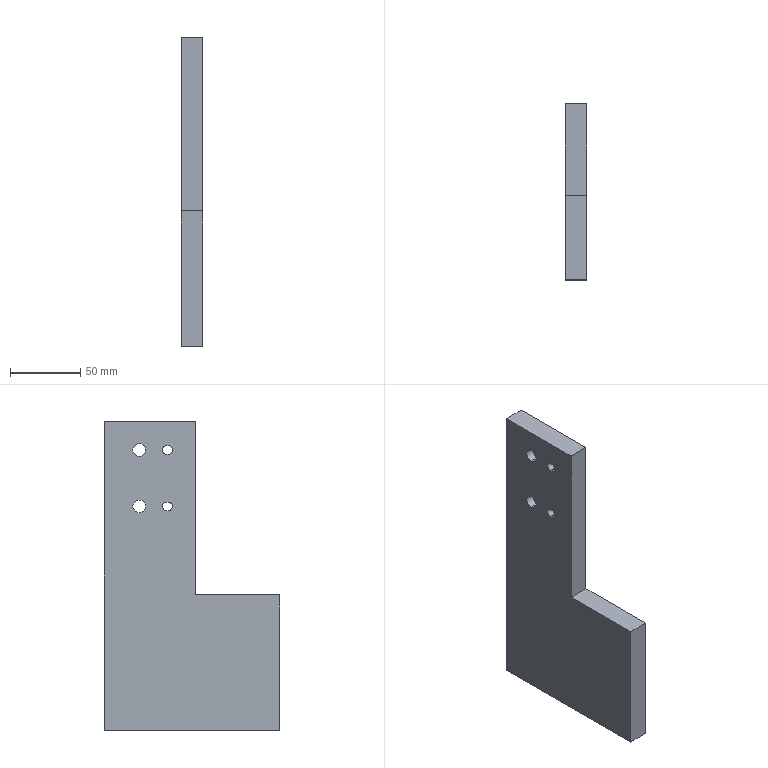Part | SolidWorks | features HoleWzd 6, Fillet 2, ICE 2, Chamfer 1, Extrusion 1 | 1 solid | 34 faces | box 15 x 125 x 219 mm | volume 294597 mm3 | cylinder 16 | plane 14 | cone 4 | commonest cylinder face diameters 4.2 x4 6 x4 9 x4 15 x4
STEP:
#1=CARTESIAN_POINT('',(2.6,-83.5,-42.9));
#2=VERTEX_POINT('',#1);
#3=CARTESIAN_POINT('',(2.6,-83.5,-47.1));
#4=VERTEX_POINT('',#3);
#5=CARTESIAN_POINT('',(2.6,-83.5,-45.));
#6=DIRECTION('',(1.,0.,0.));
#7=DIRECTION('',(0.,0.,-1.));
#8=AXIS2_PLACEMENT_3D('',#5,#6,#7);
#9=CIRCLE('',#8,2.1);
#10=EDGE_CURVE('',#2,#4,#9,.T.);
#11=ORIENTED_EDGE('',*,*,#10,.F.);
#12=CARTESIAN_POINT('',(15.,-83.5,-42.9));
#13=VERTEX_POINT('',#12);
#14=CARTESIAN_POINT('',(15.,-83.5,-42.9));
#15=DIRECTION('',(1.,0.,0.));
#16=VECTOR('',#15,1000.);
#17=LINE('',#14,#16);
#18=EDGE_CURVE('',#2,#13,#17,.T.);
#19=ORIENTED_EDGE('',*,*,#18,.T.);
#20=CARTESIAN_POINT('',(15.,-83.5,-47.1));
#21=VERTEX_POINT('',#20);
#22=CARTESIAN_POINT('',(15.,-83.5,-45.));
#23=DIRECTION('',(1.,0.,0.));
#24=DIRECTION('',(0.,0.,-1.));
#25=AXIS2_PLACEMENT_3D('',#22,#23,#24);
#26=CIRCLE('',#25,2.1);
#27=EDGE_CURVE('',#13,#21,#26,.T.);
#28=ORIENTED_EDGE('',*,*,#27,.T.);
#29=CARTESIAN_POINT('',(15.,-83.5,-47.1));
#30=DIRECTION('',(1.,0.,0.));
#31=VECTOR('',#30,1000.);
#32=LINE('',#29,#31);
#33=EDGE_CURVE('',#4,#21,#32,.T.);
#34=ORIENTED_EDGE('',*,*,#33,.F.);
#35=EDGE_LOOP('',(#11,#19,#28,#34));
#36=FACE_OUTER_BOUND('',#35,.T.);
#37=CARTESIAN_POINT('',(15.,-83.5,-45.));
#38=DIRECTION('',(1.,0.,0.));
#39=DIRECTION('',(0.,0.,-1.));
#40=AXIS2_PLACEMENT_3D('',#37,#38,#39);
#41=CYLINDRICAL_SURFACE('',#40,2.1);
#42=ADVANCED_FACE('',(#36),#41,.F.);
#43=CARTESIAN_POINT('',(1.338,-83.5,-45.));
#44=VERTEX_POINT('',#43);
#45=CARTESIAN_POINT('',(2.6,-83.5,-47.1));
#46=DIRECTION('',(0.515,0.,-0.8572));
#47=VECTOR('',#46,1000.);
#48=LINE('',#45,#47);
#49=EDGE_CURVE('',#44,#4,#48,.T.);
#50=ORIENTED_EDGE('',*,*,#49,.F.);
#51=CARTESIAN_POINT('',(2.6,-83.5,-42.9));
#52=DIRECTION('',(0.515,0.,0.8572));
#53=VECTOR('',#52,1000.);
#54=LINE('',#51,#53);
#55=EDGE_CURVE('',#44,#2,#54,.T.);
#56=ORIENTED_EDGE('',*,*,#55,.T.);
#57=ORIENTED_EDGE('',*,*,#10,.T.);
#58=EDGE_LOOP('',(#50,#56,#57));
#59=FACE_OUTER_BOUND('',#58,.T.);
#60=CARTESIAN_POINT('',(2.6,-83.5,-45.));
#61=DIRECTION('',(1.,0.,0.));
#62=DIRECTION('',(0.,0.,-1.));
#63=AXIS2_PLACEMENT_3D('',#60,#61,#62);
#64=CONICAL_SURFACE('',#63,2.1,1.03);
#65=ADVANCED_FACE('',(#59),#64,.F.);
#66=CARTESIAN_POINT('',(2.6,-83.5,-97.9));
#67=VERTEX_POINT('',#66);
#68=CARTESIAN_POINT('',(2.6,-83.5,-102.1));
#69=VERTEX_POINT('',#68);
#70=CARTESIAN_POINT('',(2.6,-83.5,-100.));
#71=DIRECTION('',(1.,0.,0.));
#72=DIRECTION('',(0.,0.,-1.));
#73=AXIS2_PLACEMENT_3D('',#70,#71,#72);
#74=CIRCLE('',#73,2.1);
#75=EDGE_CURVE('',#67,#69,#74,.T.);
#76=ORIENTED_EDGE('',*,*,#75,.F.);
#77=CARTESIAN_POINT('',(15.,-83.5,-97.9));
#78=VERTEX_POINT('',#77);
#79=CARTESIAN_POINT('',(15.,-83.5,-97.9));
#80=DIRECTION('',(1.,0.,0.));
#81=VECTOR('',#80,1000.);
#82=LINE('',#79,#81);
#83=EDGE_CURVE('',#67,#78,#82,.T.);
#84=ORIENTED_EDGE('',*,*,#83,.T.);
#85=CARTESIAN_POINT('',(15.,-83.5,-102.1));
#86=VERTEX_POINT('',#85);
#87=CARTESIAN_POINT('',(15.,-83.5,-100.));
#88=DIRECTION('',(1.,0.,0.));
#89=DIRECTION('',(0.,0.,-1.));
#90=AXIS2_PLACEMENT_3D('',#87,#88,#89);
#91=CIRCLE('',#90,2.1);
#92=EDGE_CURVE('',#78,#86,#91,.T.);
#93=ORIENTED_EDGE('',*,*,#92,.T.);
#94=CARTESIAN_POINT('',(15.,-83.5,-102.1));
#95=DIRECTION('',(1.,0.,0.));
#96=VECTOR('',#95,1000.);
#97=LINE('',#94,#96);
#98=EDGE_CURVE('',#69,#86,#97,.T.);
#99=ORIENTED_EDGE('',*,*,#98,.F.);
#100=EDGE_LOOP('',(#76,#84,#93,#99));
#101=FACE_OUTER_BOUND('',#100,.T.);
#102=CARTESIAN_POINT('',(15.,-83.5,-100.));
#103=DIRECTION('',(1.,0.,0.));
#104=DIRECTION('',(0.,0.,-1.));
#105=AXIS2_PLACEMENT_3D('',#102,#103,#104);
#106=CYLINDRICAL_SURFACE('',#105,2.1);
#107=ADVANCED_FACE('',(#101),#106,.F.);
#108=CARTESIAN_POINT('',(1.338,-83.5,-100.));
#109=VERTEX_POINT('',#108);
#110=CARTESIAN_POINT('',(2.6,-83.5,-102.1));
#111=DIRECTION('',(0.515,0.,-0.8572));
#112=VECTOR('',#111,1000.);
#113=LINE('',#110,#112);
#114=EDGE_CURVE('',#109,#69,#113,.T.);
#115=ORIENTED_EDGE('',*,*,#114,.F.);
#116=CARTESIAN_POINT('',(2.6,-83.5,-97.9));
#117=DIRECTION('',(0.515,0.,0.8572));
#118=VECTOR('',#117,1000.);
#119=LINE('',#116,#118);
#120=EDGE_CURVE('',#109,#67,#119,.T.);
#121=ORIENTED_EDGE('',*,*,#120,.T.);
#122=ORIENTED_EDGE('',*,*,#75,.T.);
#123=EDGE_LOOP('',(#115,#121,#122));
#124=FACE_OUTER_BOUND('',#123,.T.);
#125=CARTESIAN_POINT('',(2.6,-83.5,-100.));
#126=DIRECTION('',(1.,0.,0.));
#127=DIRECTION('',(0.,0.,-1.));
#128=AXIS2_PLACEMENT_3D('',#125,#126,#127);
#129=CONICAL_SURFACE('',#128,2.1,1.03);
#130=ADVANCED_FACE('',(#124),#129,.F.);
#131=CARTESIAN_POINT('',(6.,7.5,97.));
#132=VERTEX_POINT('',#131);
#133=CARTESIAN_POINT('',(6.,7.5,82.));
#134=VERTEX_POINT('',#133);
#135=CARTESIAN_POINT('',(6.,7.5,89.5));
#136=DIRECTION('',(1.,0.,0.));
#137=DIRECTION('',(0.,0.,-1.));
#138=AXIS2_PLACEMENT_3D('',#135,#136,#137);
#139=CIRCLE('',#138,7.5);
#140=EDGE_CURVE('',#132,#134,#139,.T.);
#141=ORIENTED_EDGE('',*,*,#140,.F.);
#142=CARTESIAN_POINT('',(15.,7.5,97.));
#143=VERTEX_POINT('',#142);
#144=CARTESIAN_POINT('',(15.,7.5,97.));
#145=DIRECTION('',(1.,0.,0.));
#146=VECTOR('',#145,1000.);
#147=LINE('',#144,#146);
#148=EDGE_CURVE('',#132,#143,#147,.T.);
#149=ORIENTED_EDGE('',*,*,#148,.T.);
#150=CARTESIAN_POINT('',(15.,7.5,82.));
#151=VERTEX_POINT('',#150);
#152=CARTESIAN_POINT('',(15.,7.5,89.5));
#153=DIRECTION('',(1.,0.,0.));
#154=DIRECTION('',(0.,0.,-1.));
#155=AXIS2_PLACEMENT_3D('',#152,#153,#154);
#156=CIRCLE('',#155,7.5);
#157=EDGE_CURVE('',#143,#151,#156,.T.);
#158=ORIENTED_EDGE('',*,*,#157,.T.);
#159=CARTESIAN_POINT('',(15.,7.5,82.));
#160=DIRECTION('',(1.,0.,0.));
#161=VECTOR('',#160,1000.);
#162=LINE('',#159,#161);
#163=EDGE_CURVE('',#134,#151,#162,.T.);
#164=ORIENTED_EDGE('',*,*,#163,.F.);
#165=EDGE_LOOP('',(#141,#149,#158,#164));
#166=FACE_OUTER_BOUND('',#165,.T.);
#167=CARTESIAN_POINT('',(15.,7.5,89.5));
#168=DIRECTION('',(1.,0.,0.));
#169=DIRECTION('',(0.,0.,-1.));
#170=AXIS2_PLACEMENT_3D('',#167,#168,#169);
#171=CYLINDRICAL_SURFACE('',#170,7.5);
#172=ADVANCED_FACE('',(#166),#171,.F.);
#173=CARTESIAN_POINT('',(0.,7.5,94.));
#174=VERTEX_POINT('',#173);
#175=CARTESIAN_POINT('',(0.,7.5,85.));
#176=VERTEX_POINT('',#175);
#177=CARTESIAN_POINT('',(0.,7.5,89.5));
#178=DIRECTION('',(1.,0.,0.));
#179=DIRECTION('',(0.,0.,-1.));
#180=AXIS2_PLACEMENT_3D('',#177,#178,#179);
#181=CIRCLE('',#180,4.5);
#182=EDGE_CURVE('',#174,#176,#181,.T.);
#183=ORIENTED_EDGE('',*,*,#182,.F.);
#184=CARTESIAN_POINT('',(6.,7.5,94.));
#185=VERTEX_POINT('',#184);
#186=CARTESIAN_POINT('',(15.,7.5,94.));
#187=DIRECTION('',(1.,0.,0.));
#188=VECTOR('',#187,1000.);
#189=LINE('',#186,#188);
#190=EDGE_CURVE('',#174,#185,#189,.T.);
#191=ORIENTED_EDGE('',*,*,#190,.T.);
#192=CARTESIAN_POINT('',(6.,7.5,85.));
#193=VERTEX_POINT('',#192);
#194=CARTESIAN_POINT('',(6.,7.5,89.5));
#195=DIRECTION('',(1.,0.,0.));
#196=DIRECTION('',(0.,0.,-1.));
#197=AXIS2_PLACEMENT_3D('',#194,#195,#196);
#198=CIRCLE('',#197,4.5);
#199=EDGE_CURVE('',#185,#193,#198,.T.);
#200=ORIENTED_EDGE('',*,*,#199,.T.);
#201=CARTESIAN_POINT('',(15.,7.5,85.));
#202=DIRECTION('',(1.,0.,0.));
#203=VECTOR('',#202,1000.);
#204=LINE('',#201,#203);
#205=EDGE_CURVE('',#176,#193,#204,.T.);
#206=ORIENTED_EDGE('',*,*,#205,.F.);
#207=EDGE_LOOP('',(#183,#191,#200,#206));
#208=FACE_OUTER_BOUND('',#207,.T.);
#209=CARTESIAN_POINT('',(15.,7.5,89.5));
#210=DIRECTION('',(1.,0.,0.));
#211=DIRECTION('',(0.,0.,-1.));
#212=AXIS2_PLACEMENT_3D('',#209,#210,#211);
#213=CYLINDRICAL_SURFACE('',#212,4.5);
#214=ADVANCED_FACE('',(#208),#213,.F.);
#215=CARTESIAN_POINT('',(6.,7.5,57.));
#216=VERTEX_POINT('',#215);
#217=CARTESIAN_POINT('',(6.,7.5,42.));
#218=VERTEX_POINT('',#217);
#219=CARTESIAN_POINT('',(6.,7.5,49.5));
#220=DIRECTION('',(1.,0.,0.));
#221=DIRECTION('',(0.,0.,-1.));
#222=AXIS2_PLACEMENT_3D('',#219,#220,#221);
#223=CIRCLE('',#222,7.5);
#224=EDGE_CURVE('',#216,#218,#223,.T.);
#225=ORIENTED_EDGE('',*,*,#224,.F.);
#226=CARTESIAN_POINT('',(15.,7.5,57.));
#227=VERTEX_POINT('',#226);
#228=CARTESIAN_POINT('',(15.,7.5,57.));
#229=DIRECTION('',(1.,0.,0.));
#230=VECTOR('',#229,1000.);
#231=LINE('',#228,#230);
#232=EDGE_CURVE('',#216,#227,#231,.T.);
#233=ORIENTED_EDGE('',*,*,#232,.T.);
#234=CARTESIAN_POINT('',(15.,7.5,42.));
#235=VERTEX_POINT('',#234);
#236=CARTESIAN_POINT('',(15.,7.5,49.5));
#237=DIRECTION('',(1.,0.,0.));
#238=DIRECTION('',(0.,0.,-1.));
#239=AXIS2_PLACEMENT_3D('',#236,#237,#238);
#240=CIRCLE('',#239,7.5);
#241=EDGE_CURVE('',#227,#235,#240,.T.);
#242=ORIENTED_EDGE('',*,*,#241,.T.);
#243=CARTESIAN_POINT('',(15.,7.5,42.));
#244=DIRECTION('',(1.,0.,0.));
#245=VECTOR('',#244,1000.);
#246=LINE('',#243,#245);
#247=EDGE_CURVE('',#218,#235,#246,.T.);
#248=ORIENTED_EDGE('',*,*,#247,.F.);
#249=EDGE_LOOP('',(#225,#233,#242,#248));
#250=FACE_OUTER_BOUND('',#249,.T.);
#251=CARTESIAN_POINT('',(15.,7.5,49.5));
#252=DIRECTION('',(1.,0.,0.));
#253=DIRECTION('',(0.,0.,-1.));
#254=AXIS2_PLACEMENT_3D('',#251,#252,#253);
#255=CYLINDRICAL_SURFACE('',#254,7.5);
#256=ADVANCED_FACE('',(#250),#255,.F.);
#257=CARTESIAN_POINT('',(0.,7.5,54.));
#258=VERTEX_POINT('',#257);
#259=CARTESIAN_POINT('',(0.,7.5,45.));
#260=VERTEX_POINT('',#259);
#261=CARTESIAN_POINT('',(0.,7.5,49.5));
#262=DIRECTION('',(1.,0.,0.));
#263=DIRECTION('',(0.,0.,-1.));
#264=AXIS2_PLACEMENT_3D('',#261,#262,#263);
#265=CIRCLE('',#264,4.5);
#266=EDGE_CURVE('',#258,#260,#265,.T.);
#267=ORIENTED_EDGE('',*,*,#266,.F.);
#268=CARTESIAN_POINT('',(6.,7.5,54.));
#269=VERTEX_POINT('',#268);
#270=CARTESIAN_POINT('',(15.,7.5,54.));
#271=DIRECTION('',(1.,0.,0.));
#272=VECTOR('',#271,1000.);
#273=LINE('',#270,#272);
#274=EDGE_CURVE('',#258,#269,#273,.T.);
#275=ORIENTED_EDGE('',*,*,#274,.T.);
#276=CARTESIAN_POINT('',(6.,7.5,45.));
#277=VERTEX_POINT('',#276);
#278=CARTESIAN_POINT('',(6.,7.5,49.5));
#279=DIRECTION('',(1.,0.,0.));
#280=DIRECTION('',(0.,0.,-1.));
#281=AXIS2_PLACEMENT_3D('',#278,#279,#280);
#282=CIRCLE('',#281,4.5);
#283=EDGE_CURVE('',#269,#277,#282,.T.);
#284=ORIENTED_EDGE('',*,*,#283,.T.);
#285=CARTESIAN_POINT('',(15.,7.5,45.));
#286=DIRECTION('',(1.,0.,0.));
#287=VECTOR('',#286,1000.);
#288=LINE('',#285,#287);
#289=EDGE_CURVE('',#260,#277,#288,.T.);
#290=ORIENTED_EDGE('',*,*,#289,.F.);
#291=EDGE_LOOP('',(#267,#275,#284,#290));
#292=FACE_OUTER_BOUND('',#291,.T.);
#293=CARTESIAN_POINT('',(15.,7.5,49.5));
#294=DIRECTION('',(1.,0.,0.));
#295=DIRECTION('',(0.,0.,-1.));
#296=AXIS2_PLACEMENT_3D('',#293,#294,#295);
#297=CYLINDRICAL_SURFACE('',#296,4.5);
#298=ADVANCED_FACE('',(#292),#297,.F.);
#299=CARTESIAN_POINT('',(15.,-32.5,-13.5));
#300=VERTEX_POINT('',#299);
#301=CARTESIAN_POINT('',(0.,-32.5,-13.5));
#302=VERTEX_POINT('',#301);
#303=CARTESIAN_POINT('',(0.,-32.5,-13.5));
#304=DIRECTION('',(-1.,0.,0.));
#305=VECTOR('',#304,1000.);
#306=LINE('',#303,#305);
#307=EDGE_CURVE('',#300,#302,#306,.T.);
#308=ORIENTED_EDGE('',*,*,#307,.F.);
#309=CARTESIAN_POINT('',(15.,-32.5,109.5));
#310=VERTEX_POINT('',#309);
#311=CARTESIAN_POINT('',(15.,-32.5,109.5));
#312=DIRECTION('',(0.,0.,-1.));
#313=VECTOR('',#312,1000.);
#314=LINE('',#311,#313);
#315=EDGE_CURVE('',#310,#300,#314,.T.);
#316=ORIENTED_EDGE('',*,*,#315,.F.);
#317=CARTESIAN_POINT('',(0.,-32.5,109.5));
#318=VERTEX_POINT('',#317);
#319=CARTESIAN_POINT('',(15.,-32.5,109.5));
#320=DIRECTION('',(-1.,0.,0.));
#321=VECTOR('',#320,1000.);
#322=LINE('',#319,#321);
#323=EDGE_CURVE('',#310,#318,#322,.T.);
#324=ORIENTED_EDGE('',*,*,#323,.T.);
#325=CARTESIAN_POINT('',(0.,-32.5,109.5));
#326=DIRECTION('',(0.,0.,-1.));
#327=VECTOR('',#326,1000.);
#328=LINE('',#325,#327);
#329=EDGE_CURVE('',#318,#302,#328,.T.);
#330=ORIENTED_EDGE('',*,*,#329,.T.);
#331=EDGE_LOOP('',(#308,#316,#324,#330));
#332=FACE_OUTER_BOUND('',#331,.T.);
#333=CARTESIAN_POINT('',(15.,-32.5,109.5));
#334=DIRECTION('',(0.,1.,0.));
#335=DIRECTION('',(0.,0.,1.));
#336=AXIS2_PLACEMENT_3D('',#333,#334,#335);
#337=PLANE('',#336);
#338=ADVANCED_FACE('',(#332),#337,.F.);
#339=CARTESIAN_POINT('',(15.,-83.5,-45.));
#340=DIRECTION('',(1.,0.,0.));
#341=DIRECTION('',(0.,0.,-1.));
#342=AXIS2_PLACEMENT_3D('',#339,#340,#341);
#343=CIRCLE('',#342,2.1);
#344=EDGE_CURVE('',#21,#13,#343,.T.);
#345=ORIENTED_EDGE('',*,*,#344,.F.);
#346=ORIENTED_EDGE('',*,*,#27,.F.);
#347=EDGE_LOOP('',(#345,#346));
#348=FACE_BOUND('',#347,.T.);
#349=CARTESIAN_POINT('',(15.,-83.5,-100.));
#350=DIRECTION('',(1.,0.,0.));
#351=DIRECTION('',(0.,0.,-1.));
#352=AXIS2_PLACEMENT_3D('',#349,#350,#351);
#353=CIRCLE('',#352,2.1);
#354=EDGE_CURVE('',#86,#78,#353,.T.);
#355=ORIENTED_EDGE('',*,*,#354,.F.);
#356=ORIENTED_EDGE('',*,*,#92,.F.);
#357=EDGE_LOOP('',(#355,#356));
#358=FACE_BOUND('',#357,.T.);
#359=CARTESIAN_POINT('',(15.,-92.5,-109.5));
#360=VERTEX_POINT('',#359);
#361=CARTESIAN_POINT('',(15.,32.5,-109.5));
#362=VERTEX_POINT('',#361);
#363=CARTESIAN_POINT('',(15.,-32.5,-109.5));
#364=DIRECTION('',(0.,1.,0.));
#365=VECTOR('',#364,1000.);
#366=LINE('',#363,#365);
#367=EDGE_CURVE('',#360,#362,#366,.T.);
#368=ORIENTED_EDGE('',*,*,#367,.T.);
#369=CARTESIAN_POINT('',(15.,32.5,109.5));
#370=VERTEX_POINT('',#369);
#371=CARTESIAN_POINT('',(15.,32.5,109.5));
#372=DIRECTION('',(0.,0.,1.));
#373=VECTOR('',#372,1000.);
#374=LINE('',#371,#373);
#375=EDGE_CURVE('',#362,#370,#374,.T.);
#376=ORIENTED_EDGE('',*,*,#375,.T.);
#377=CARTESIAN_POINT('',(15.,-32.5,109.5));
#378=DIRECTION('',(0.,-1.,0.));
#379=VECTOR('',#378,1000.);
#380=LINE('',#377,#379);
#381=EDGE_CURVE('',#370,#310,#380,.T.);
#382=ORIENTED_EDGE('',*,*,#381,.T.);
#383=ORIENTED_EDGE('',*,*,#315,.T.);
#384=CARTESIAN_POINT('',(15.,-92.5,-13.5));
#385=VERTEX_POINT('',#384);
#386=CARTESIAN_POINT('',(15.,-92.5,-13.5));
#387=DIRECTION('',(0.,1.,0.));
#388=VECTOR('',#387,1000.);
#389=LINE('',#386,#388);
#390=EDGE_CURVE('',#385,#300,#389,.T.);
#391=ORIENTED_EDGE('',*,*,#390,.F.);
#392=CARTESIAN_POINT('',(15.,-92.5,-109.5));
#393=DIRECTION('',(0.,0.,1.));
#394=VECTOR('',#393,1000.);
#395=LINE('',#392,#394);
#396=EDGE_CURVE('',#360,#385,#395,.T.);
#397=ORIENTED_EDGE('',*,*,#396,.F.);
#398=EDGE_LOOP('',(#368,#376,#382,#383,#391,#397));
#399=FACE_OUTER_BOUND('',#398,.T.);
#400=CARTESIAN_POINT('',(15.,7.5,49.5));
#401=DIRECTION('',(1.,0.,0.));
#402=DIRECTION('',(0.,0.,-1.));
#403=AXIS2_PLACEMENT_3D('',#400,#401,#402);
#404=CIRCLE('',#403,7.5);
#405=EDGE_CURVE('',#235,#227,#404,.T.);
#406=ORIENTED_EDGE('',*,*,#405,.F.);
#407=ORIENTED_EDGE('',*,*,#241,.F.);
#408=EDGE_LOOP('',(#406,#407));
#409=FACE_BOUND('',#408,.T.);
#410=CARTESIAN_POINT('',(15.,7.5,89.5));
#411=DIRECTION('',(1.,0.,0.));
#412=DIRECTION('',(0.,0.,-1.));
#413=AXIS2_PLACEMENT_3D('',#410,#411,#412);
#414=CIRCLE('',#413,7.5);
#415=EDGE_CURVE('',#151,#143,#414,.T.);
#416=ORIENTED_EDGE('',*,*,#415,.F.);
#417=ORIENTED_EDGE('',*,*,#157,.F.);
#418=EDGE_LOOP('',(#416,#417));
#419=FACE_BOUND('',#418,.T.);
#420=CARTESIAN_POINT('',(15.,-13.,52.5));
#421=VERTEX_POINT('',#420);
#422=CARTESIAN_POINT('',(15.,-13.,46.5));
#423=VERTEX_POINT('',#422);
#424=CARTESIAN_POINT('',(15.,-13.,49.5));
#425=DIRECTION('',(1.,0.,0.));
#426=DIRECTION('',(0.,0.,-1.));
#427=AXIS2_PLACEMENT_3D('',#424,#425,#426);
#428=CIRCLE('',#427,3.);
#429=EDGE_CURVE('',#421,#423,#428,.T.);
#430=ORIENTED_EDGE('',*,*,#429,.F.);
#431=CARTESIAN_POINT('',(15.,-12.,52.5));
#432=VERTEX_POINT('',#431);
#433=CARTESIAN_POINT('',(15.,-13.,52.5));
#434=DIRECTION('',(0.,1.,0.));
#435=VECTOR('',#434,1000.);
#436=LINE('',#433,#435);
#437=EDGE_CURVE('',#421,#432,#436,.T.);
#438=ORIENTED_EDGE('',*,*,#437,.T.);
#439=CARTESIAN_POINT('',(15.,-12.,46.5));
#440=VERTEX_POINT('',#439);
#441=CARTESIAN_POINT('',(15.,-12.,49.5));
#442=DIRECTION('',(1.,0.,0.));
#443=DIRECTION('',(0.,0.,-1.));
#444=AXIS2_PLACEMENT_3D('',#441,#442,#443);
#445=CIRCLE('',#444,3.);
#446=EDGE_CURVE('',#440,#432,#445,.T.);
#447=ORIENTED_EDGE('',*,*,#446,.F.);
#448=CARTESIAN_POINT('',(15.,-13.,46.5));
#449=DIRECTION('',(0.,1.,0.));
#450=VECTOR('',#449,1000.);
#451=LINE('',#448,#450);
#452=EDGE_CURVE('',#423,#440,#451,.T.);
#453=ORIENTED_EDGE('',*,*,#452,.F.);
#454=EDGE_LOOP('',(#430,#438,#447,#453));
#455=FACE_BOUND('',#454,.T.);
#456=CARTESIAN_POINT('',(15.,-12.,86.5));
#457=VERTEX_POINT('',#456);
#458=CARTESIAN_POINT('',(15.,-12.,92.5));
#459=VERTEX_POINT('',#458);
#460=CARTESIAN_POINT('',(15.,-12.,89.5));
#461=DIRECTION('',(1.,0.,0.));
#462=DIRECTION('',(0.,0.,-1.));
#463=AXIS2_PLACEMENT_3D('',#460,#461,#462);
#464=CIRCLE('',#463,3.);
#465=EDGE_CURVE('',#457,#459,#464,.T.);
#466=ORIENTED_EDGE('',*,*,#465,.F.);
#467=CARTESIAN_POINT('',(15.,-13.,86.5));
#468=VERTEX_POINT('',#467);
#469=CARTESIAN_POINT('',(15.,-13.,86.5));
#470=DIRECTION('',(0.,1.,0.));
#471=VECTOR('',#470,1000.);
#472=LINE('',#469,#471);
#473=EDGE_CURVE('',#468,#457,#472,.T.);
#474=ORIENTED_EDGE('',*,*,#473,.F.);
#475=CARTESIAN_POINT('',(15.,-13.,92.5));
#476=VERTEX_POINT('',#475);
#477=CARTESIAN_POINT('',(15.,-13.,89.5));
#478=DIRECTION('',(1.,0.,0.));
#479=DIRECTION('',(0.,0.,-1.));
#480=AXIS2_PLACEMENT_3D('',#477,#478,#479);
#481=CIRCLE('',#480,3.);
#482=EDGE_CURVE('',#476,#468,#481,.T.);
#483=ORIENTED_EDGE('',*,*,#482,.F.);
#484=CARTESIAN_POINT('',(15.,-13.,92.5));
#485=DIRECTION('',(0.,1.,0.));
#486=VECTOR('',#485,1000.);
#487=LINE('',#484,#486);
#488=EDGE_CURVE('',#476,#459,#487,.T.);
#489=ORIENTED_EDGE('',*,*,#488,.T.);
#490=EDGE_LOOP('',(#466,#474,#483,#489));
#491=FACE_BOUND('',#490,.T.);
#492=CARTESIAN_POINT('',(15.,0.,0.));
#493=DIRECTION('',(-1.,0.,0.));
#494=DIRECTION('',(0.,0.,1.));
#495=AXIS2_PLACEMENT_3D('',#492,#493,#494);
#496=PLANE('',#495);
#497=ADVANCED_FACE('',(#348,#358,#399,#409,#419,#455,#491),#496,.F.);
#498=CARTESIAN_POINT('',(0.,-13.,46.5));
#499=VERTEX_POINT('',#498);
#500=CARTESIAN_POINT('',(0.,-12.,46.5));
#501=VERTEX_POINT('',#500);
#502=CARTESIAN_POINT('',(0.,-13.,46.5));
#503=DIRECTION('',(0.,1.,0.));
#504=VECTOR('',#503,1000.);
#505=LINE('',#502,#504);
#506=EDGE_CURVE('',#499,#501,#505,.T.);
#507=ORIENTED_EDGE('',*,*,#506,.T.);
#508=CARTESIAN_POINT('',(0.,-12.,52.5));
#509=VERTEX_POINT('',#508);
#510=CARTESIAN_POINT('',(0.,-12.,49.5));
#511=DIRECTION('',(1.,0.,0.));
#512=DIRECTION('',(0.,0.,-1.));
#513=AXIS2_PLACEMENT_3D('',#510,#511,#512);
#514=CIRCLE('',#513,3.);
#515=EDGE_CURVE('',#501,#509,#514,.T.);
#516=ORIENTED_EDGE('',*,*,#515,.T.);
#517=CARTESIAN_POINT('',(0.,-13.,52.5));
#518=VERTEX_POINT('',#517);
#519=CARTESIAN_POINT('',(0.,-13.,52.5));
#520=DIRECTION('',(0.,1.,0.));
#521=VECTOR('',#520,1000.);
#522=LINE('',#519,#521);
#523=EDGE_CURVE('',#518,#509,#522,.T.);
#524=ORIENTED_EDGE('',*,*,#523,.F.);
#525=CARTESIAN_POINT('',(0.,-13.,49.5));
#526=DIRECTION('',(1.,0.,0.));
#527=DIRECTION('',(0.,0.,-1.));
#528=AXIS2_PLACEMENT_3D('',#525,#526,#527);
#529=CIRCLE('',#528,3.);
#530=EDGE_CURVE('',#518,#499,#529,.T.);
#531=ORIENTED_EDGE('',*,*,#530,.T.);
#532=EDGE_LOOP('',(#507,#516,#524,#531));
#533=FACE_BOUND('',#532,.T.);
#534=CARTESIAN_POINT('',(0.,7.5,89.5));
#535=DIRECTION('',(1.,0.,0.));
#536=DIRECTION('',(0.,0.,-1.));
#537=AXIS2_PLACEMENT_3D('',#534,#535,#536);
#538=CIRCLE('',#537,4.5);
#539=EDGE_CURVE('',#176,#174,#538,.T.);
#540=ORIENTED_EDGE('',*,*,#539,.T.);
#541=ORIENTED_EDGE('',*,*,#182,.T.);
#542=EDGE_LOOP('',(#540,#541));
#543=FACE_BOUND('',#542,.T.);
#544=CARTESIAN_POINT('',(0.,7.5,49.5));
#545=DIRECTION('',(1.,0.,0.));
#546=DIRECTION('',(0.,0.,-1.));
#547=AXIS2_PLACEMENT_3D('',#544,#545,#546);
#548=CIRCLE('',#547,4.5);
#549=EDGE_CURVE('',#260,#258,#548,.T.);
#550=ORIENTED_EDGE('',*,*,#549,.T.);
#551=ORIENTED_EDGE('',*,*,#266,.T.);
#552=EDGE_LOOP('',(#550,#551));
#553=FACE_BOUND('',#552,.T.);
#554=CARTESIAN_POINT('',(0.,-92.5,-109.5));
#555=VERTEX_POINT('',#554);
#556=CARTESIAN_POINT('',(0.,32.5,-109.5));
#557=VERTEX_POINT('',#556);
#558=CARTESIAN_POINT('',(0.,-32.5,-109.5));
#559=DIRECTION('',(0.,1.,0.));
#560=VECTOR('',#559,1000.);
#561=LINE('',#558,#560);
#562=EDGE_CURVE('',#555,#557,#561,.T.);
#563=ORIENTED_EDGE('',*,*,#562,.F.);
#564=CARTESIAN_POINT('',(0.,-92.5,-13.5));
#565=VERTEX_POINT('',#564);
#566=CARTESIAN_POINT('',(0.,-92.5,-109.5));
#567=DIRECTION('',(0.,0.,-1.));
#568=VECTOR('',#567,1000.);
#569=LINE('',#566,#568);
#570=EDGE_CURVE('',#565,#555,#569,.T.);
#571=ORIENTED_EDGE('',*,*,#570,.F.);
#572=CARTESIAN_POINT('',(0.,-92.5,-13.5));
#573=DIRECTION('',(0.,1.,0.));
#574=VECTOR('',#573,1000.);
#575=LINE('',#572,#574);
#576=EDGE_CURVE('',#565,#302,#575,.T.);
#577=ORIENTED_EDGE('',*,*,#576,.T.);
#578=ORIENTED_EDGE('',*,*,#329,.F.);
#579=CARTESIAN_POINT('',(0.,32.5,109.5));
#580=VERTEX_POINT('',#579);
#581=CARTESIAN_POINT('',(0.,-32.5,109.5));
#582=DIRECTION('',(0.,-1.,0.));
#583=VECTOR('',#582,1000.);
#584=LINE('',#581,#583);
#585=EDGE_CURVE('',#580,#318,#584,.T.);
#586=ORIENTED_EDGE('',*,*,#585,.F.);
#587=CARTESIAN_POINT('',(0.,32.5,109.5));
#588=DIRECTION('',(0.,0.,1.));
#589=VECTOR('',#588,1000.);
#590=LINE('',#587,#589);
#591=EDGE_CURVE('',#557,#580,#590,.T.);
#592=ORIENTED_EDGE('',*,*,#591,.F.);
#593=EDGE_LOOP('',(#563,#571,#577,#578,#586,#592));
#594=FACE_OUTER_BOUND('',#593,.T.);
#595=CARTESIAN_POINT('',(0.,-13.,86.5));
#596=VERTEX_POINT('',#595);
#597=CARTESIAN_POINT('',(0.,-12.,86.5));
#598=VERTEX_POINT('',#597);
#599=CARTESIAN_POINT('',(0.,-13.,86.5));
#600=DIRECTION('',(0.,1.,0.));
#601=VECTOR('',#600,1000.);
#602=LINE('',#599,#601);
#603=EDGE_CURVE('',#596,#598,#602,.T.);
#604=ORIENTED_EDGE('',*,*,#603,.T.);
#605=CARTESIAN_POINT('',(0.,-12.,92.5));
#606=VERTEX_POINT('',#605);
#607=CARTESIAN_POINT('',(0.,-12.,89.5));
#608=DIRECTION('',(1.,0.,0.));
#609=DIRECTION('',(0.,0.,-1.));
#610=AXIS2_PLACEMENT_3D('',#607,#608,#609);
#611=CIRCLE('',#610,3.);
#612=EDGE_CURVE('',#598,#606,#611,.T.);
#613=ORIENTED_EDGE('',*,*,#612,.T.);
#614=CARTESIAN_POINT('',(0.,-13.,92.5));
#615=VERTEX_POINT('',#614);
#616=CARTESIAN_POINT('',(0.,-13.,92.5));
#617=DIRECTION('',(0.,1.,0.));
#618=VECTOR('',#617,1000.);
#619=LINE('',#616,#618);
#620=EDGE_CURVE('',#615,#606,#619,.T.);
#621=ORIENTED_EDGE('',*,*,#620,.F.);
#622=CARTESIAN_POINT('',(0.,-13.,89.5));
#623=DIRECTION('',(1.,0.,0.));
#624=DIRECTION('',(0.,0.,-1.));
#625=AXIS2_PLACEMENT_3D('',#622,#623,#624);
#626=CIRCLE('',#625,3.);
#627=EDGE_CURVE('',#615,#596,#626,.T.);
#628=ORIENTED_EDGE('',*,*,#627,.T.);
#629=EDGE_LOOP('',(#604,#613,#621,#628));
#630=FACE_BOUND('',#629,.T.);
#631=CARTESIAN_POINT('',(0.,0.,0.));
#632=DIRECTION('',(-1.,0.,0.));
#633=DIRECTION('',(0.,0.,1.));
#634=AXIS2_PLACEMENT_3D('',#631,#632,#633);
#635=PLANE('',#634);
#636=ADVANCED_FACE('',(#533,#543,#553,#594,#630),#635,.T.);
#637=ORIENTED_EDGE('',*,*,#562,.T.);
#638=CARTESIAN_POINT('',(15.,32.5,-109.5));
#639=DIRECTION('',(-1.,0.,0.));
#640=VECTOR('',#639,1000.);
#641=LINE('',#638,#640);
#642=EDGE_CURVE('',#362,#557,#641,.T.);
#643=ORIENTED_EDGE('',*,*,#642,.F.);
#644=ORIENTED_EDGE('',*,*,#367,.F.);
#645=CARTESIAN_POINT('',(0.,-92.5,-109.5));
#646=DIRECTION('',(1.,0.,0.));
#647=VECTOR('',#646,1000.);
#648=LINE('',#645,#647);
#649=EDGE_CURVE('',#555,#360,#648,.T.);
#650=ORIENTED_EDGE('',*,*,#649,.F.);
#651=EDGE_LOOP('',(#637,#643,#644,#650));
#652=FACE_OUTER_BOUND('',#651,.T.);
#653=CARTESIAN_POINT('',(15.,-32.5,-109.5));
#654=DIRECTION('',(0.,0.,1.));
#655=DIRECTION('',(1.,0.,0.));
#656=AXIS2_PLACEMENT_3D('',#653,#654,#655);
#657=PLANE('',#656);
#658=ADVANCED_FACE('',(#652),#657,.F.);
#659=ORIENTED_EDGE('',*,*,#591,.T.);
#660=CARTESIAN_POINT('',(15.,32.5,109.5));
#661=DIRECTION('',(-1.,0.,0.));
#662=VECTOR('',#661,1000.);
#663=LINE('',#660,#662);
#664=EDGE_CURVE('',#370,#580,#663,.T.);
#665=ORIENTED_EDGE('',*,*,#664,.F.);
#666=ORIENTED_EDGE('',*,*,#375,.F.);
#667=ORIENTED_EDGE('',*,*,#642,.T.);
#668=EDGE_LOOP('',(#659,#665,#666,#667));
#669=FACE_OUTER_BOUND('',#668,.T.);
#670=CARTESIAN_POINT('',(15.,32.5,109.5));
#671=DIRECTION('',(0.,-1.,0.));
#672=DIRECTION('',(0.,0.,-1.));
#673=AXIS2_PLACEMENT_3D('',#670,#671,#672);
#674=PLANE('',#673);
#675=ADVANCED_FACE('',(#669),#674,.F.);
#676=ORIENTED_EDGE('',*,*,#585,.T.);
#677=ORIENTED_EDGE('',*,*,#323,.F.);
#678=ORIENTED_EDGE('',*,*,#381,.F.);
#679=ORIENTED_EDGE('',*,*,#664,.T.);
#680=EDGE_LOOP('',(#676,#677,#678,#679));
#681=FACE_OUTER_BOUND('',#680,.T.);
#682=CARTESIAN_POINT('',(15.,-32.5,109.5));
#683=DIRECTION('',(0.,0.,-1.));
#684=DIRECTION('',(-1.,0.,0.));
#685=AXIS2_PLACEMENT_3D('',#682,#683,#684);
#686=PLANE('',#685);
#687=ADVANCED_FACE('',(#681),#686,.F.);
#688=ORIENTED_EDGE('',*,*,#274,.F.);
#689=ORIENTED_EDGE('',*,*,#549,.F.);
#690=ORIENTED_EDGE('',*,*,#289,.T.);
#691=CARTESIAN_POINT('',(6.,7.5,49.5));
#692=DIRECTION('',(1.,0.,0.));
#693=DIRECTION('',(0.,0.,-1.));
#694=AXIS2_PLACEMENT_3D('',#691,#692,#693);
#695=CIRCLE('',#694,4.5);
#696=EDGE_CURVE('',#277,#269,#695,.T.);
#697=ORIENTED_EDGE('',*,*,#696,.T.);
#698=EDGE_LOOP('',(#688,#689,#690,#697));
#699=FACE_OUTER_BOUND('',#698,.T.);
#700=CARTESIAN_POINT('',(15.,7.5,49.5));
#701=DIRECTION('',(1.,0.,0.));
#702=DIRECTION('',(0.,0.,-1.));
#703=AXIS2_PLACEMENT_3D('',#700,#701,#702);
#704=CYLINDRICAL_SURFACE('',#703,4.5);
#705=ADVANCED_FACE('',(#699),#704,.F.);
#706=ORIENTED_EDGE('',*,*,#696,.F.);
#707=ORIENTED_EDGE('',*,*,#283,.F.);
#708=EDGE_LOOP('',(#706,#707));
#709=FACE_BOUND('',#708,.T.);
#710=CARTESIAN_POINT('',(6.,7.5,49.5));
#711=DIRECTION('',(1.,0.,0.));
#712=DIRECTION('',(0.,0.,-1.));
#713=AXIS2_PLACEMENT_3D('',#710,#711,#712);
#714=CIRCLE('',#713,7.5);
#715=EDGE_CURVE('',#218,#216,#714,.T.);
#716=ORIENTED_EDGE('',*,*,#715,.T.);
#717=ORIENTED_EDGE('',*,*,#224,.T.);
#718=EDGE_LOOP('',(#716,#717));
#719=FACE_OUTER_BOUND('',#718,.T.);
#720=CARTESIAN_POINT('',(6.,12.,49.5));
#721=DIRECTION('',(-1.,0.,0.));
#722=DIRECTION('',(0.,0.,1.));
#723=AXIS2_PLACEMENT_3D('',#720,#721,#722);
#724=PLANE('',#723);
#725=ADVANCED_FACE('',(#709,#719),#724,.F.);
#726=ORIENTED_EDGE('',*,*,#232,.F.);
#727=ORIENTED_EDGE('',*,*,#715,.F.);
#728=ORIENTED_EDGE('',*,*,#247,.T.);
#729=ORIENTED_EDGE('',*,*,#405,.T.);
#730=EDGE_LOOP('',(#726,#727,#728,#729));
#731=FACE_OUTER_BOUND('',#730,.T.);
#732=CARTESIAN_POINT('',(15.,7.5,49.5));
#733=DIRECTION('',(1.,0.,0.));
#734=DIRECTION('',(0.,0.,-1.));
#735=AXIS2_PLACEMENT_3D('',#732,#733,#734);
#736=CYLINDRICAL_SURFACE('',#735,7.5);
#737=ADVANCED_FACE('',(#731),#736,.F.);
#738=ORIENTED_EDGE('',*,*,#190,.F.);
#739=ORIENTED_EDGE('',*,*,#539,.F.);
#740=ORIENTED_EDGE('',*,*,#205,.T.);
#741=CARTESIAN_POINT('',(6.,7.5,89.5));
#742=DIRECTION('',(1.,0.,0.));
#743=DIRECTION('',(0.,0.,-1.));
#744=AXIS2_PLACEMENT_3D('',#741,#742,#743);
#745=CIRCLE('',#744,4.5);
#746=EDGE_CURVE('',#193,#185,#745,.T.);
#747=ORIENTED_EDGE('',*,*,#746,.T.);
#748=EDGE_LOOP('',(#738,#739,#740,#747));
#749=FACE_OUTER_BOUND('',#748,.T.);
#750=CARTESIAN_POINT('',(15.,7.5,89.5));
#751=DIRECTION('',(1.,0.,0.));
#752=DIRECTION('',(0.,0.,-1.));
#753=AXIS2_PLACEMENT_3D('',#750,#751,#752);
#754=CYLINDRICAL_SURFACE('',#753,4.5);
#755=ADVANCED_FACE('',(#749),#754,.F.);
#756=ORIENTED_EDGE('',*,*,#746,.F.);
#757=ORIENTED_EDGE('',*,*,#199,.F.);
#758=EDGE_LOOP('',(#756,#757));
#759=FACE_BOUND('',#758,.T.);
#760=CARTESIAN_POINT('',(6.,7.5,89.5));
#761=DIRECTION('',(1.,0.,0.));
#762=DIRECTION('',(0.,0.,-1.));
#763=AXIS2_PLACEMENT_3D('',#760,#761,#762);
#764=CIRCLE('',#763,7.5);
#765=EDGE_CURVE('',#134,#132,#764,.T.);
#766=ORIENTED_EDGE('',*,*,#765,.T.);
#767=ORIENTED_EDGE('',*,*,#140,.T.);
#768=EDGE_LOOP('',(#766,#767));
#769=FACE_OUTER_BOUND('',#768,.T.);
#770=CARTESIAN_POINT('',(6.,12.,89.5));
#771=DIRECTION('',(-1.,0.,0.));
#772=DIRECTION('',(0.,0.,1.));
#773=AXIS2_PLACEMENT_3D('',#770,#771,#772);
#774=PLANE('',#773);
#775=ADVANCED_FACE('',(#759,#769),#774,.F.);
#776=ORIENTED_EDGE('',*,*,#148,.F.);
#777=ORIENTED_EDGE('',*,*,#765,.F.);
#778=ORIENTED_EDGE('',*,*,#163,.T.);
#779=ORIENTED_EDGE('',*,*,#415,.T.);
#780=EDGE_LOOP('',(#776,#777,#778,#779));
#781=FACE_OUTER_BOUND('',#780,.T.);
#782=CARTESIAN_POINT('',(15.,7.5,89.5));
#783=DIRECTION('',(1.,0.,0.));
#784=DIRECTION('',(0.,0.,-1.));
#785=AXIS2_PLACEMENT_3D('',#782,#783,#784);
#786=CYLINDRICAL_SURFACE('',#785,7.5);
#787=ADVANCED_FACE('',(#781),#786,.F.);
#788=ORIENTED_EDGE('',*,*,#515,.F.);
#789=CARTESIAN_POINT('',(15.,-12.,46.5));
#790=DIRECTION('',(-1.,0.,0.));
#791=VECTOR('',#790,1000.);
#792=LINE('',#789,#791);
#793=EDGE_CURVE('',#440,#501,#792,.T.);
#794=ORIENTED_EDGE('',*,*,#793,.F.);
#795=ORIENTED_EDGE('',*,*,#446,.T.);
#796=CARTESIAN_POINT('',(15.,-12.,52.5));
#797=DIRECTION('',(1.,0.,0.));
#798=VECTOR('',#797,1000.);
#799=LINE('',#796,#798);
#800=EDGE_CURVE('',#509,#432,#799,.T.);
#801=ORIENTED_EDGE('',*,*,#800,.F.);
#802=EDGE_LOOP('',(#788,#794,#795,#801));
#803=FACE_OUTER_BOUND('',#802,.T.);
#804=CARTESIAN_POINT('',(15.,-12.,49.5));
#805=DIRECTION('',(1.,0.,0.));
#806=DIRECTION('',(0.,0.,-1.));
#807=AXIS2_PLACEMENT_3D('',#804,#805,#806);
#808=CYLINDRICAL_SURFACE('',#807,3.);
#809=ADVANCED_FACE('',(#803),#808,.F.);
#810=ORIENTED_EDGE('',*,*,#429,.T.);
#811=CARTESIAN_POINT('',(15.,-13.,46.5));
#812=DIRECTION('',(1.,0.,0.));
#813=VECTOR('',#812,1000.);
#814=LINE('',#811,#813);
#815=EDGE_CURVE('',#499,#423,#814,.T.);
#816=ORIENTED_EDGE('',*,*,#815,.F.);
#817=ORIENTED_EDGE('',*,*,#530,.F.);
#818=CARTESIAN_POINT('',(15.,-13.,52.5));
#819=DIRECTION('',(-1.,0.,0.));
#820=VECTOR('',#819,1000.);
#821=LINE('',#818,#820);
#822=EDGE_CURVE('',#421,#518,#821,.T.);
#823=ORIENTED_EDGE('',*,*,#822,.F.);
#824=EDGE_LOOP('',(#810,#816,#817,#823));
#825=FACE_OUTER_BOUND('',#824,.T.);
#826=CARTESIAN_POINT('',(15.,-13.,49.5));
#827=DIRECTION('',(1.,0.,0.));
#828=DIRECTION('',(0.,0.,-1.));
#829=AXIS2_PLACEMENT_3D('',#826,#827,#828);
#830=CYLINDRICAL_SURFACE('',#829,3.);
#831=ADVANCED_FACE('',(#825),#830,.F.);
#832=ORIENTED_EDGE('',*,*,#800,.T.);
#833=ORIENTED_EDGE('',*,*,#437,.F.);
#834=ORIENTED_EDGE('',*,*,#822,.T.);
#835=ORIENTED_EDGE('',*,*,#523,.T.);
#836=EDGE_LOOP('',(#832,#833,#834,#835));
#837=FACE_OUTER_BOUND('',#836,.T.);
#838=CARTESIAN_POINT('',(15.,-13.,52.5));
#839=DIRECTION('',(0.,0.,1.));
#840=DIRECTION('',(1.,0.,0.));
#841=AXIS2_PLACEMENT_3D('',#838,#839,#840);
#842=PLANE('',#841);
#843=ADVANCED_FACE('',(#837),#842,.F.);
#844=ORIENTED_EDGE('',*,*,#793,.T.);
#845=ORIENTED_EDGE('',*,*,#506,.F.);
#846=ORIENTED_EDGE('',*,*,#815,.T.);
#847=ORIENTED_EDGE('',*,*,#452,.T.);
#848=EDGE_LOOP('',(#844,#845,#846,#847));
#849=FACE_OUTER_BOUND('',#848,.T.);
#850=CARTESIAN_POINT('',(15.,-13.,46.5));
#851=DIRECTION('',(0.,0.,-1.));
#852=DIRECTION('',(-1.,0.,0.));
#853=AXIS2_PLACEMENT_3D('',#850,#851,#852);
#854=PLANE('',#853);
#855=ADVANCED_FACE('',(#849),#854,.F.);
#856=ORIENTED_EDGE('',*,*,#612,.F.);
#857=CARTESIAN_POINT('',(15.,-12.,86.5));
#858=DIRECTION('',(-1.,0.,0.));
#859=VECTOR('',#858,1000.);
#860=LINE('',#857,#859);
#861=EDGE_CURVE('',#457,#598,#860,.T.);
#862=ORIENTED_EDGE('',*,*,#861,.F.);
#863=ORIENTED_EDGE('',*,*,#465,.T.);
#864=CARTESIAN_POINT('',(15.,-12.,92.5));
#865=DIRECTION('',(1.,0.,0.));
#866=VECTOR('',#865,1000.);
#867=LINE('',#864,#866);
#868=EDGE_CURVE('',#606,#459,#867,.T.);
#869=ORIENTED_EDGE('',*,*,#868,.F.);
#870=EDGE_LOOP('',(#856,#862,#863,#869));
#871=FACE_OUTER_BOUND('',#870,.T.);
#872=CARTESIAN_POINT('',(15.,-12.,89.5));
#873=DIRECTION('',(1.,0.,0.));
#874=DIRECTION('',(0.,0.,-1.));
#875=AXIS2_PLACEMENT_3D('',#872,#873,#874);
#876=CYLINDRICAL_SURFACE('',#875,3.);
#877=ADVANCED_FACE('',(#871),#876,.F.);
#878=ORIENTED_EDGE('',*,*,#482,.T.);
#879=CARTESIAN_POINT('',(15.,-13.,86.5));
#880=DIRECTION('',(1.,0.,0.));
#881=VECTOR('',#880,1000.);
#882=LINE('',#879,#881);
#883=EDGE_CURVE('',#596,#468,#882,.T.);
#884=ORIENTED_EDGE('',*,*,#883,.F.);
#885=ORIENTED_EDGE('',*,*,#627,.F.);
#886=CARTESIAN_POINT('',(15.,-13.,92.5));
#887=DIRECTION('',(-1.,0.,0.));
#888=VECTOR('',#887,1000.);
#889=LINE('',#886,#888);
#890=EDGE_CURVE('',#476,#615,#889,.T.);
#891=ORIENTED_EDGE('',*,*,#890,.F.);
#892=EDGE_LOOP('',(#878,#884,#885,#891));
#893=FACE_OUTER_BOUND('',#892,.T.);
#894=CARTESIAN_POINT('',(15.,-13.,89.5));
#895=DIRECTION('',(1.,0.,0.));
#896=DIRECTION('',(0.,0.,-1.));
#897=AXIS2_PLACEMENT_3D('',#894,#895,#896);
#898=CYLINDRICAL_SURFACE('',#897,3.);
#899=ADVANCED_FACE('',(#893),#898,.F.);
#900=ORIENTED_EDGE('',*,*,#868,.T.);
#901=ORIENTED_EDGE('',*,*,#488,.F.);
#902=ORIENTED_EDGE('',*,*,#890,.T.);
#903=ORIENTED_EDGE('',*,*,#620,.T.);
#904=EDGE_LOOP('',(#900,#901,#902,#903));
#905=FACE_OUTER_BOUND('',#904,.T.);
#906=CARTESIAN_POINT('',(15.,-13.,92.5));
#907=DIRECTION('',(0.,0.,1.));
#908=DIRECTION('',(1.,0.,0.));
#909=AXIS2_PLACEMENT_3D('',#906,#907,#908);
#910=PLANE('',#909);
#911=ADVANCED_FACE('',(#905),#910,.F.);
#912=ORIENTED_EDGE('',*,*,#861,.T.);
#913=ORIENTED_EDGE('',*,*,#603,.F.);
#914=ORIENTED_EDGE('',*,*,#883,.T.);
#915=ORIENTED_EDGE('',*,*,#473,.T.);
#916=EDGE_LOOP('',(#912,#913,#914,#915));
#917=FACE_OUTER_BOUND('',#916,.T.);
#918=CARTESIAN_POINT('',(15.,-13.,86.5));
#919=DIRECTION('',(0.,0.,-1.));
#920=DIRECTION('',(-1.,0.,0.));
#921=AXIS2_PLACEMENT_3D('',#918,#919,#920);
#922=PLANE('',#921);
#923=ADVANCED_FACE('',(#917),#922,.F.);
#924=ORIENTED_EDGE('',*,*,#307,.T.);
#925=ORIENTED_EDGE('',*,*,#576,.F.);
#926=CARTESIAN_POINT('',(0.,-92.5,-13.5));
#927=DIRECTION('',(-1.,0.,0.));
#928=VECTOR('',#927,1000.);
#929=LINE('',#926,#928);
#930=EDGE_CURVE('',#385,#565,#929,.T.);
#931=ORIENTED_EDGE('',*,*,#930,.F.);
#932=ORIENTED_EDGE('',*,*,#390,.T.);
#933=EDGE_LOOP('',(#924,#925,#931,#932));
#934=FACE_OUTER_BOUND('',#933,.T.);
#935=CARTESIAN_POINT('',(0.,-92.5,-13.5));
#936=DIRECTION('',(0.,0.,-1.));
#937=DIRECTION('',(-1.,0.,0.));
#938=AXIS2_PLACEMENT_3D('',#935,#936,#937);
#939=PLANE('',#938);
#940=ADVANCED_FACE('',(#934),#939,.F.);
#941=ORIENTED_EDGE('',*,*,#570,.T.);
#942=ORIENTED_EDGE('',*,*,#649,.T.);
#943=ORIENTED_EDGE('',*,*,#396,.T.);
#944=ORIENTED_EDGE('',*,*,#930,.T.);
#945=EDGE_LOOP('',(#941,#942,#943,#944));
#946=FACE_OUTER_BOUND('',#945,.T.);
#947=CARTESIAN_POINT('',(0.,-92.5,0.));
#948=DIRECTION('',(0.,1.,0.));
#949=DIRECTION('',(0.,0.,1.));
#950=AXIS2_PLACEMENT_3D('',#947,#948,#949);
#951=PLANE('',#950);
#952=ADVANCED_FACE('',(#946),#951,.F.);
#953=ORIENTED_EDGE('',*,*,#120,.F.);
#954=ORIENTED_EDGE('',*,*,#114,.T.);
#955=CARTESIAN_POINT('',(2.6,-83.5,-100.));
#956=DIRECTION('',(1.,0.,0.));
#957=DIRECTION('',(0.,0.,-1.));
#958=AXIS2_PLACEMENT_3D('',#955,#956,#957);
#959=CIRCLE('',#958,2.1);
#960=EDGE_CURVE('',#69,#67,#959,.T.);
#961=ORIENTED_EDGE('',*,*,#960,.T.);
#962=EDGE_LOOP('',(#953,#954,#961));
#963=FACE_OUTER_BOUND('',#962,.T.);
#964=CARTESIAN_POINT('',(2.6,-83.5,-100.));
#965=DIRECTION('',(1.,0.,0.));
#966=DIRECTION('',(0.,0.,-1.));
#967=AXIS2_PLACEMENT_3D('',#964,#965,#966);
#968=CONICAL_SURFACE('',#967,2.1,1.03);
#969=ADVANCED_FACE('',(#963),#968,.F.);
#970=ORIENTED_EDGE('',*,*,#83,.F.);
#971=ORIENTED_EDGE('',*,*,#960,.F.);
#972=ORIENTED_EDGE('',*,*,#98,.T.);
#973=ORIENTED_EDGE('',*,*,#354,.T.);
#974=EDGE_LOOP('',(#970,#971,#972,#973));
#975=FACE_OUTER_BOUND('',#974,.T.);
#976=CARTESIAN_POINT('',(15.,-83.5,-100.));
#977=DIRECTION('',(1.,0.,0.));
#978=DIRECTION('',(0.,0.,-1.));
#979=AXIS2_PLACEMENT_3D('',#976,#977,#978);
#980=CYLINDRICAL_SURFACE('',#979,2.1);
#981=ADVANCED_FACE('',(#975),#980,.F.);
#982=ORIENTED_EDGE('',*,*,#55,.F.);
#983=ORIENTED_EDGE('',*,*,#49,.T.);
#984=CARTESIAN_POINT('',(2.6,-83.5,-45.));
#985=DIRECTION('',(1.,0.,0.));
#986=DIRECTION('',(0.,0.,-1.));
#987=AXIS2_PLACEMENT_3D('',#984,#985,#986);
#988=CIRCLE('',#987,2.1);
#989=EDGE_CURVE('',#4,#2,#988,.T.);
#990=ORIENTED_EDGE('',*,*,#989,.T.);
#991=EDGE_LOOP('',(#982,#983,#990));
#992=FACE_OUTER_BOUND('',#991,.T.);
#993=CARTESIAN_POINT('',(2.6,-83.5,-45.));
#994=DIRECTION('',(1.,0.,0.));
#995=DIRECTION('',(0.,0.,-1.));
#996=AXIS2_PLACEMENT_3D('',#993,#994,#995);
#997=CONICAL_SURFACE('',#996,2.1,1.03);
#998=ADVANCED_FACE('',(#992),#997,.F.);
#999=ORIENTED_EDGE('',*,*,#18,.F.);
#1000=ORIENTED_EDGE('',*,*,#989,.F.);
#1001=ORIENTED_EDGE('',*,*,#33,.T.);
#1002=ORIENTED_EDGE('',*,*,#344,.T.);
#1003=EDGE_LOOP('',(#999,#1000,#1001,#1002));
#1004=FACE_OUTER_BOUND('',#1003,.T.);
#1005=CARTESIAN_POINT('',(15.,-83.5,-45.));
#1006=DIRECTION('',(1.,0.,0.));
#1007=DIRECTION('',(0.,0.,-1.));
#1008=AXIS2_PLACEMENT_3D('',#1005,#1006,#1007);
#1009=CYLINDRICAL_SURFACE('',#1008,2.1);
#1010=ADVANCED_FACE('',(#1004),#1009,.F.);
#1011=CLOSED_SHELL('',(#42,#65,#107,#130,#172,#214,#256,#298,#338,#497,#636,#658,#675,#687,#705,#725,#737,#755,#775,#787,#809,#831,#843,#855,#877,#899,#911,#923,#940,#952,#969,#981,#998,#1010));
#1012=MANIFOLD_SOLID_BREP('',#1011);
#1013=CARTESIAN_POINT('',(0.,0.,0.));
#1014=DIRECTION('',(0.,0.,1.));
#1015=DIRECTION('',(1.,0.,0.));
#1016=AXIS2_PLACEMENT_3D('',#1013,#1014,#1015);
#1017=(LENGTH_UNIT()NAMED_UNIT(*)SI_UNIT(.MILLI.,.METRE.));
#1018=UNCERTAINTY_MEASURE_WITH_UNIT(LENGTH_MEASURE(0.00001),#1017,'','');
#1019=(NAMED_UNIT(*)PLANE_ANGLE_UNIT()SI_UNIT($,.RADIAN.));
#1020=(NAMED_UNIT(*)SI_UNIT($,.STERADIAN.)SOLID_ANGLE_UNIT());
#1021=(GEOMETRIC_REPRESENTATION_CONTEXT(3)GLOBAL_UNCERTAINTY_ASSIGNED_CONTEXT((#1018))GLOBAL_UNIT_ASSIGNED_CONTEXT((#1017,#1019,#1020))REPRESENTATION_CONTEXT('',''));
#1022=ADVANCED_BREP_SHAPE_REPRESENTATION('',(#1012,#1016),#1021);